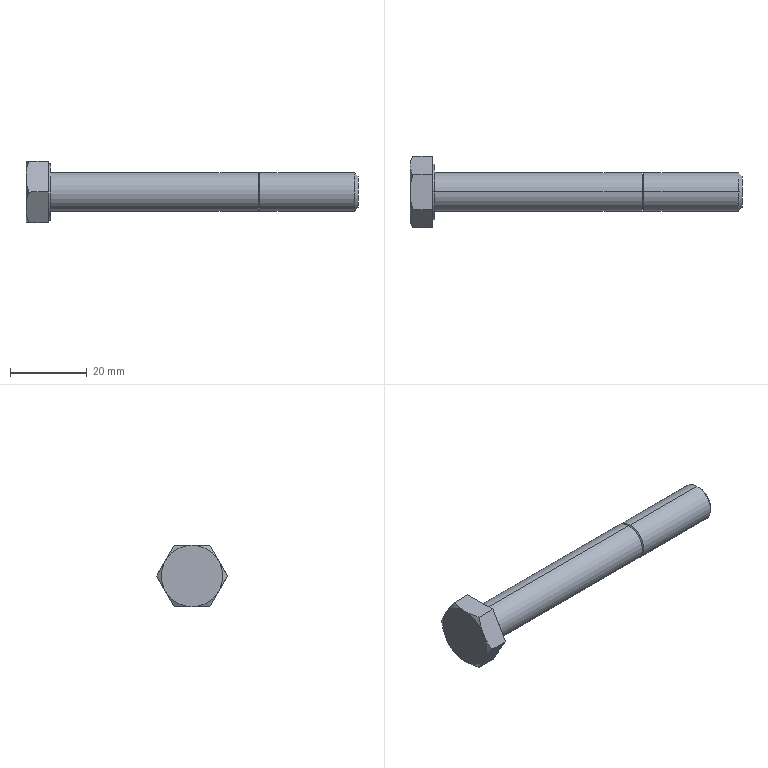Part | STEP file | HEX-HEAD BOLT - KS B 1002 - A M10X80.stp | 1 solid | 23 faces | box 86.4 x 18.48 x 16 mm | volume 7648 mm3 | plane 11 | cone 6 | cylinder 6 | commonest cylinder face diameters 10 x4 14.63 x2